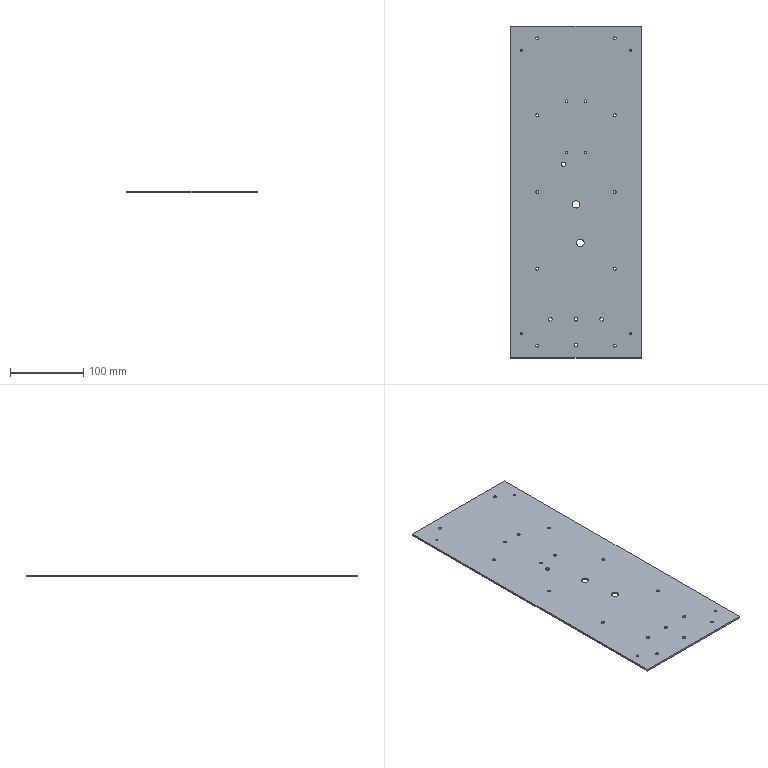Part | STEP file | 1-43.1 | 1 solid | 31 faces | box 178 x 454 x 2.5 mm | volume 200860 mm3 | cylinder 25 | plane 6 | commonest cylinder face diameters 4 x14 3 x4 5 x4 10 x2 6 x1